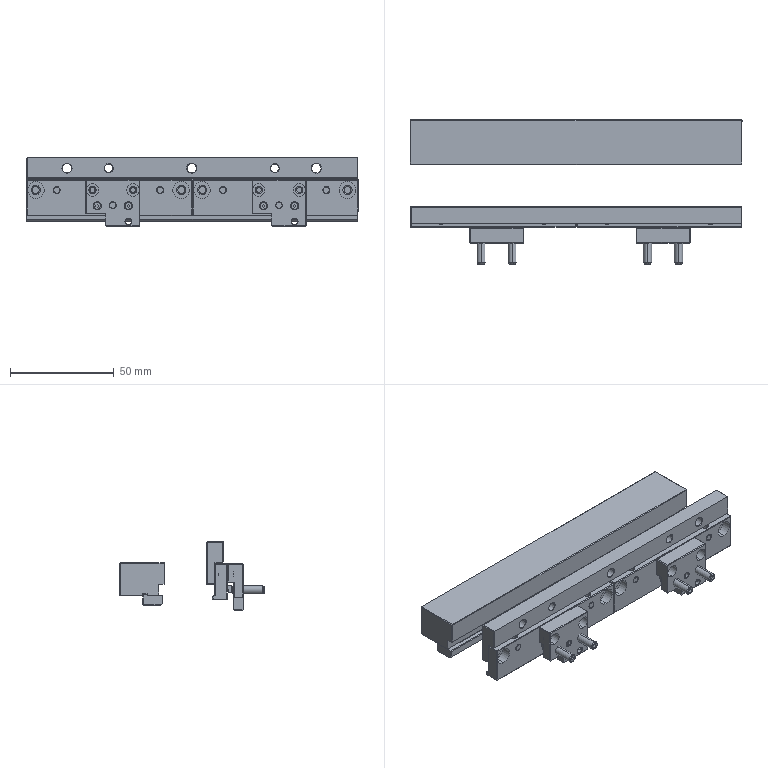Part | NX | 19 solids | 596 faces | box 159.75 x 69.305 x 32.9 mm | volume 98844 mm3 | plane 288 | cylinder 188 | cone 114 | sphere 6 | commonest cylinder face diameters 2.5 x36 3 x34 3.3 x28 4 x16 3.5 x14 4.5 x14